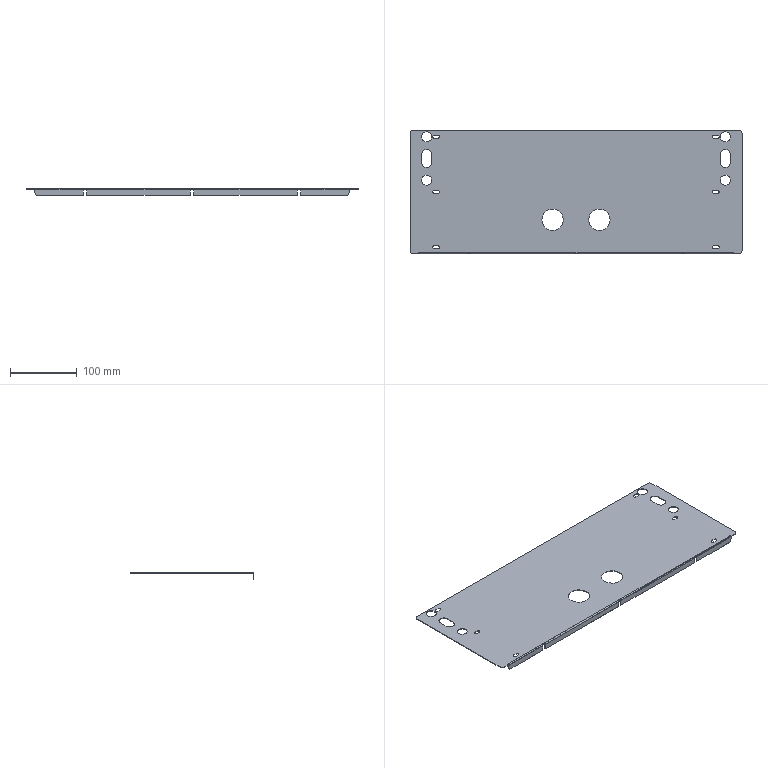Part | SolidWorks | features Cut 2, HoleWzd 2, BreakCorner 1, EdgeFlange 1, FlatPattern 1, ICE 1, SMBaseFlange 1, SheetMetal 1 | 1 solid | 96 faces | box 496 x 185 x 10 mm | volume 92290 mm3 | plane 54 | cylinder 42 | commonest cylinder face diameters 4.8 x18 15 x12 10 x6 32 x4 1.473 x1 3.473 x1